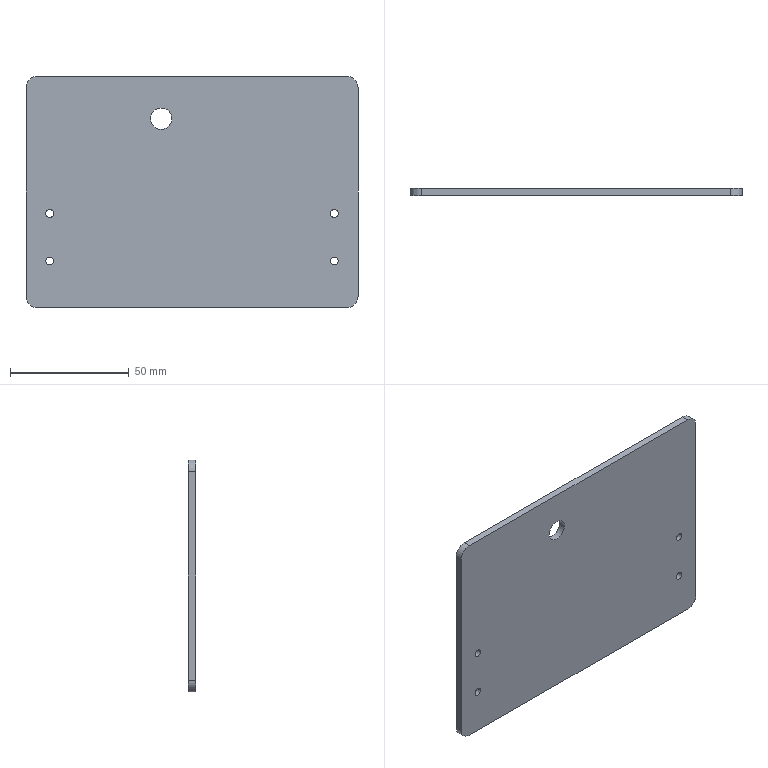Part | NX | 1 solid | 30 faces | box 140 x 3 x 97.8 mm | volume 40712 mm3 | cylinder 14 | cone 10 | plane 6 | commonest cylinder face diameters 3.3 x8 10 x4 9 x2
STEP:
#1=CARTESIAN_POINT('',(1167.,-112.5,-32.3));
#2=VERTEX_POINT('',#1);
#3=CARTESIAN_POINT('',(1167.,-109.5,-32.3));
#4=VERTEX_POINT('',#3);
#5=CARTESIAN_POINT('',(1167.,-112.5,-32.3));
#6=DIRECTION('',(0.,1.,0.));
#7=VECTOR('',#6,1000.);
#8=LINE('',#5,#7);
#9=EDGE_CURVE('',#2,#4,#8,.T.);
#10=ORIENTED_EDGE('',*,*,#9,.F.);
#11=CARTESIAN_POINT('',(1167.,-112.5,55.5));
#12=VERTEX_POINT('',#11);
#13=CARTESIAN_POINT('',(1167.,-112.5,40.233));
#14=DIRECTION('',(0.,0.,1.));
#15=VECTOR('',#14,1000.);
#16=LINE('',#13,#15);
#17=EDGE_CURVE('',#2,#12,#16,.T.);
#18=ORIENTED_EDGE('',*,*,#17,.T.);
#19=CARTESIAN_POINT('',(1167.,-109.5,55.5));
#20=VERTEX_POINT('',#19);
#21=CARTESIAN_POINT('',(1167.,-112.5,55.5));
#22=DIRECTION('',(0.,1.,0.));
#23=VECTOR('',#22,1000.);
#24=LINE('',#21,#23);
#25=EDGE_CURVE('',#12,#20,#24,.T.);
#26=ORIENTED_EDGE('',*,*,#25,.T.);
#27=CARTESIAN_POINT('',(1167.,-109.5,40.233));
#28=DIRECTION('',(0.,0.,1.));
#29=VECTOR('',#28,1000.);
#30=LINE('',#27,#29);
#31=EDGE_CURVE('',#4,#20,#30,.T.);
#32=ORIENTED_EDGE('',*,*,#31,.F.);
#33=EDGE_LOOP('',(#10,#18,#26,#32));
#34=FACE_BOUND('',#33,.T.);
#35=CARTESIAN_POINT('',(1167.,-112.5,22.3));
#36=DIRECTION('',(-1.,0.,0.));
#37=DIRECTION('',(0.,0.,1.));
#38=AXIS2_PLACEMENT_3D('',#35,#36,#37);
#39=PLANE('',#38);
#40=ADVANCED_FACE('',(#34),#39,.T.);
#41=CARTESIAN_POINT('',(1302.,-109.5,60.5));
#42=VERTEX_POINT('',#41);
#43=CARTESIAN_POINT('',(1302.,-112.5,60.5));
#44=VERTEX_POINT('',#43);
#45=CARTESIAN_POINT('',(1302.,-112.5,60.5));
#46=DIRECTION('',(0.,-1.,0.));
#47=VECTOR('',#46,1000.);
#48=LINE('',#45,#47);
#49=EDGE_CURVE('',#42,#44,#48,.T.);
#50=ORIENTED_EDGE('',*,*,#49,.F.);
#51=CARTESIAN_POINT('',(1172.,-109.5,60.5));
#52=VERTEX_POINT('',#51);
#53=CARTESIAN_POINT('',(1169.667,-109.5,60.5));
#54=DIRECTION('',(1.,0.,0.));
#55=VECTOR('',#54,1000.);
#56=LINE('',#53,#55);
#57=EDGE_CURVE('',#52,#42,#56,.T.);
#58=ORIENTED_EDGE('',*,*,#57,.F.);
#59=CARTESIAN_POINT('',(1172.,-112.5,60.5));
#60=VERTEX_POINT('',#59);
#61=CARTESIAN_POINT('',(1172.,-112.5,60.5));
#62=DIRECTION('',(0.,1.,0.));
#63=VECTOR('',#62,1000.);
#64=LINE('',#61,#63);
#65=EDGE_CURVE('',#60,#52,#64,.T.);
#66=ORIENTED_EDGE('',*,*,#65,.F.);
#67=CARTESIAN_POINT('',(1169.667,-112.5,60.5));
#68=DIRECTION('',(1.,0.,0.));
#69=VECTOR('',#68,1000.);
#70=LINE('',#67,#69);
#71=EDGE_CURVE('',#60,#44,#70,.T.);
#72=ORIENTED_EDGE('',*,*,#71,.T.);
#73=EDGE_LOOP('',(#50,#58,#66,#72));
#74=FACE_BOUND('',#73,.T.);
#75=CARTESIAN_POINT('',(1307.,-112.5,60.5));
#76=DIRECTION('',(0.,0.,1.));
#77=DIRECTION('',(1.,0.,0.));
#78=AXIS2_PLACEMENT_3D('',#75,#76,#77);
#79=PLANE('',#78);
#80=ADVANCED_FACE('',(#74),#79,.T.);
#81=CARTESIAN_POINT('',(1307.,-112.5,-32.3));
#82=VERTEX_POINT('',#81);
#83=CARTESIAN_POINT('',(1307.,-109.5,-32.3));
#84=VERTEX_POINT('',#83);
#85=CARTESIAN_POINT('',(1307.,-112.5,-32.3));
#86=DIRECTION('',(0.,1.,0.));
#87=VECTOR('',#86,1000.);
#88=LINE('',#85,#87);
#89=EDGE_CURVE('',#82,#84,#88,.T.);
#90=ORIENTED_EDGE('',*,*,#89,.T.);
#91=CARTESIAN_POINT('',(1307.,-109.5,55.5));
#92=VERTEX_POINT('',#91);
#93=CARTESIAN_POINT('',(1307.,-109.5,40.233));
#94=DIRECTION('',(0.,0.,1.));
#95=VECTOR('',#94,1000.);
#96=LINE('',#93,#95);
#97=EDGE_CURVE('',#84,#92,#96,.T.);
#98=ORIENTED_EDGE('',*,*,#97,.T.);
#99=CARTESIAN_POINT('',(1307.,-112.5,55.5));
#100=VERTEX_POINT('',#99);
#101=CARTESIAN_POINT('',(1307.,-112.5,55.5));
#102=DIRECTION('',(0.,-1.,0.));
#103=VECTOR('',#102,1000.);
#104=LINE('',#101,#103);
#105=EDGE_CURVE('',#92,#100,#104,.T.);
#106=ORIENTED_EDGE('',*,*,#105,.T.);
#107=CARTESIAN_POINT('',(1307.,-112.5,40.233));
#108=DIRECTION('',(0.,0.,1.));
#109=VECTOR('',#108,1000.);
#110=LINE('',#107,#109);
#111=EDGE_CURVE('',#82,#100,#110,.T.);
#112=ORIENTED_EDGE('',*,*,#111,.F.);
#113=EDGE_LOOP('',(#90,#98,#106,#112));
#114=FACE_BOUND('',#113,.T.);
#115=CARTESIAN_POINT('',(1307.,-112.5,-37.3));
#116=DIRECTION('',(1.,0.,0.));
#117=DIRECTION('',(0.,1.,0.));
#118=AXIS2_PLACEMENT_3D('',#115,#116,#117);
#119=PLANE('',#118);
#120=ADVANCED_FACE('',(#114),#119,.T.);
#121=CARTESIAN_POINT('',(1302.,-112.5,-37.3));
#122=VERTEX_POINT('',#121);
#123=CARTESIAN_POINT('',(1172.,-112.5,-37.3));
#124=VERTEX_POINT('',#123);
#125=CARTESIAN_POINT('',(1307.,-112.5,-37.3));
#126=DIRECTION('',(-1.,0.,0.));
#127=VECTOR('',#126,1000.);
#128=LINE('',#125,#127);
#129=EDGE_CURVE('',#122,#124,#128,.T.);
#130=ORIENTED_EDGE('',*,*,#129,.T.);
#131=CARTESIAN_POINT('',(1172.,-109.5,-37.3));
#132=VERTEX_POINT('',#131);
#133=CARTESIAN_POINT('',(1172.,-112.5,-37.3));
#134=DIRECTION('',(0.,1.,0.));
#135=VECTOR('',#134,1000.);
#136=LINE('',#133,#135);
#137=EDGE_CURVE('',#124,#132,#136,.T.);
#138=ORIENTED_EDGE('',*,*,#137,.T.);
#139=CARTESIAN_POINT('',(1302.,-109.5,-37.3));
#140=VERTEX_POINT('',#139);
#141=CARTESIAN_POINT('',(1307.,-109.5,-37.3));
#142=DIRECTION('',(-1.,0.,0.));
#143=VECTOR('',#142,1000.);
#144=LINE('',#141,#143);
#145=EDGE_CURVE('',#140,#132,#144,.T.);
#146=ORIENTED_EDGE('',*,*,#145,.F.);
#147=CARTESIAN_POINT('',(1302.,-112.5,-37.3));
#148=DIRECTION('',(0.,1.,0.));
#149=VECTOR('',#148,1000.);
#150=LINE('',#147,#149);
#151=EDGE_CURVE('',#122,#140,#150,.T.);
#152=ORIENTED_EDGE('',*,*,#151,.F.);
#153=EDGE_LOOP('',(#130,#138,#146,#152));
#154=FACE_BOUND('',#153,.T.);
#155=CARTESIAN_POINT('',(1167.,-112.5,-37.3));
#156=DIRECTION('',(0.,0.,-1.));
#157=DIRECTION('',(0.,-1.,0.));
#158=AXIS2_PLACEMENT_3D('',#155,#156,#157);
#159=PLANE('',#158);
#160=ADVANCED_FACE('',(#154),#159,.T.);
#161=ORIENTED_EDGE('',*,*,#25,.F.);
#162=CARTESIAN_POINT('',(1172.,-112.5,55.5));
#163=DIRECTION('',(0.,1.,0.));
#164=DIRECTION('',(-1.,0.,0.));
#165=AXIS2_PLACEMENT_3D('',#162,#163,#164);
#166=CIRCLE('',#165,5.);
#167=EDGE_CURVE('',#12,#60,#166,.T.);
#168=ORIENTED_EDGE('',*,*,#167,.T.);
#169=ORIENTED_EDGE('',*,*,#65,.T.);
#170=CARTESIAN_POINT('',(1172.,-109.5,55.5));
#171=DIRECTION('',(0.,1.,0.));
#172=DIRECTION('',(-1.,0.,0.));
#173=AXIS2_PLACEMENT_3D('',#170,#171,#172);
#174=CIRCLE('',#173,5.);
#175=EDGE_CURVE('',#20,#52,#174,.T.);
#176=ORIENTED_EDGE('',*,*,#175,.F.);
#177=EDGE_LOOP('',(#161,#168,#169,#176));
#178=FACE_BOUND('',#177,.T.);
#179=CARTESIAN_POINT('',(1172.,-112.5,55.5));
#180=DIRECTION('',(0.,1.,0.));
#181=DIRECTION('',(-1.,0.,0.));
#182=AXIS2_PLACEMENT_3D('',#179,#180,#181);
#183=CYLINDRICAL_SURFACE('',#182,5.);
#184=ADVANCED_FACE('',(#178),#183,.T.);
#185=ORIENTED_EDGE('',*,*,#49,.T.);
#186=CARTESIAN_POINT('',(1302.,-112.5,55.5));
#187=DIRECTION('',(0.,-1.,0.));
#188=DIRECTION('',(1.,0.,0.));
#189=AXIS2_PLACEMENT_3D('',#186,#187,#188);
#190=CIRCLE('',#189,5.);
#191=EDGE_CURVE('',#100,#44,#190,.T.);
#192=ORIENTED_EDGE('',*,*,#191,.F.);
#193=ORIENTED_EDGE('',*,*,#105,.F.);
#194=CARTESIAN_POINT('',(1302.,-109.5,55.5));
#195=DIRECTION('',(0.,-1.,0.));
#196=DIRECTION('',(1.,0.,0.));
#197=AXIS2_PLACEMENT_3D('',#194,#195,#196);
#198=CIRCLE('',#197,5.);
#199=EDGE_CURVE('',#92,#42,#198,.T.);
#200=ORIENTED_EDGE('',*,*,#199,.T.);
#201=EDGE_LOOP('',(#185,#192,#193,#200));
#202=FACE_BOUND('',#201,.T.);
#203=CARTESIAN_POINT('',(1302.,-112.5,55.5));
#204=DIRECTION('',(0.,-1.,0.));
#205=DIRECTION('',(1.,0.,0.));
#206=AXIS2_PLACEMENT_3D('',#203,#204,#205);
#207=CYLINDRICAL_SURFACE('',#206,5.);
#208=ADVANCED_FACE('',(#202),#207,.T.);
#209=ORIENTED_EDGE('',*,*,#89,.F.);
#210=CARTESIAN_POINT('',(1302.,-112.5,-32.3));
#211=DIRECTION('',(0.,1.,0.));
#212=DIRECTION('',(-1.,0.,0.));
#213=AXIS2_PLACEMENT_3D('',#210,#211,#212);
#214=CIRCLE('',#213,5.);
#215=EDGE_CURVE('',#82,#122,#214,.T.);
#216=ORIENTED_EDGE('',*,*,#215,.T.);
#217=ORIENTED_EDGE('',*,*,#151,.T.);
#218=CARTESIAN_POINT('',(1302.,-109.5,-32.3));
#219=DIRECTION('',(0.,1.,0.));
#220=DIRECTION('',(-1.,0.,0.));
#221=AXIS2_PLACEMENT_3D('',#218,#219,#220);
#222=CIRCLE('',#221,5.);
#223=EDGE_CURVE('',#84,#140,#222,.T.);
#224=ORIENTED_EDGE('',*,*,#223,.F.);
#225=EDGE_LOOP('',(#209,#216,#217,#224));
#226=FACE_BOUND('',#225,.T.);
#227=CARTESIAN_POINT('',(1302.,-112.5,-32.3));
#228=DIRECTION('',(0.,1.,0.));
#229=DIRECTION('',(-1.,0.,0.));
#230=AXIS2_PLACEMENT_3D('',#227,#228,#229);
#231=CYLINDRICAL_SURFACE('',#230,5.);
#232=ADVANCED_FACE('',(#226),#231,.T.);
#233=ORIENTED_EDGE('',*,*,#9,.T.);
#234=CARTESIAN_POINT('',(1172.,-109.5,-32.3));
#235=DIRECTION('',(0.,1.,0.));
#236=DIRECTION('',(-1.,0.,0.));
#237=AXIS2_PLACEMENT_3D('',#234,#235,#236);
#238=CIRCLE('',#237,5.);
#239=EDGE_CURVE('',#132,#4,#238,.T.);
#240=ORIENTED_EDGE('',*,*,#239,.F.);
#241=ORIENTED_EDGE('',*,*,#137,.F.);
#242=CARTESIAN_POINT('',(1172.,-112.5,-32.3));
#243=DIRECTION('',(0.,1.,0.));
#244=DIRECTION('',(-1.,0.,0.));
#245=AXIS2_PLACEMENT_3D('',#242,#243,#244);
#246=CIRCLE('',#245,5.);
#247=EDGE_CURVE('',#124,#2,#246,.T.);
#248=ORIENTED_EDGE('',*,*,#247,.T.);
#249=EDGE_LOOP('',(#233,#240,#241,#248));
#250=FACE_BOUND('',#249,.T.);
#251=CARTESIAN_POINT('',(1172.,-112.5,-32.3));
#252=DIRECTION('',(0.,1.,0.));
#253=DIRECTION('',(-1.,0.,0.));
#254=AXIS2_PLACEMENT_3D('',#251,#252,#253);
#255=CYLINDRICAL_SURFACE('',#254,5.);
#256=ADVANCED_FACE('',(#250),#255,.T.);
#257=CARTESIAN_POINT('',(1178.65,-109.884,-17.5));
#258=VERTEX_POINT('',#257);
#259=CARTESIAN_POINT('',(1175.35,-109.884,-17.5));
#260=VERTEX_POINT('',#259);
#261=CARTESIAN_POINT('',(1177.,-109.884,-17.5));
#262=DIRECTION('',(0.,1.,0.));
#263=DIRECTION('',(-1.,0.,0.));
#264=AXIS2_PLACEMENT_3D('',#261,#262,#263);
#265=CIRCLE('',#264,1.65);
#266=EDGE_CURVE('',#258,#260,#265,.T.);
#267=ORIENTED_EDGE('',*,*,#266,.T.);
#268=CARTESIAN_POINT('',(1175.35,-112.5,-17.5));
#269=VERTEX_POINT('',#268);
#270=CARTESIAN_POINT('',(1175.35,-109.5,-17.5));
#271=DIRECTION('',(0.,1.,0.));
#272=VECTOR('',#271,1000.);
#273=LINE('',#270,#272);
#274=EDGE_CURVE('',#260,#269,#273,.F.);
#275=ORIENTED_EDGE('',*,*,#274,.T.);
#276=CARTESIAN_POINT('',(1178.65,-112.5,-17.5));
#277=VERTEX_POINT('',#276);
#278=CARTESIAN_POINT('',(1177.,-112.5,-17.5));
#279=DIRECTION('',(0.,1.,0.));
#280=DIRECTION('',(-1.,0.,0.));
#281=AXIS2_PLACEMENT_3D('',#278,#279,#280);
#282=CIRCLE('',#281,1.65);
#283=EDGE_CURVE('',#277,#269,#282,.T.);
#284=ORIENTED_EDGE('',*,*,#283,.F.);
#285=CARTESIAN_POINT('',(1178.65,-109.5,-17.5));
#286=DIRECTION('',(0.,1.,0.));
#287=VECTOR('',#286,1000.);
#288=LINE('',#285,#287);
#289=EDGE_CURVE('',#258,#277,#288,.F.);
#290=ORIENTED_EDGE('',*,*,#289,.F.);
#291=EDGE_LOOP('',(#267,#275,#284,#290));
#292=FACE_BOUND('',#291,.T.);
#293=CARTESIAN_POINT('',(1177.,-109.5,-17.5));
#294=DIRECTION('',(0.,1.,0.));
#295=DIRECTION('',(-1.,0.,0.));
#296=AXIS2_PLACEMENT_3D('',#293,#294,#295);
#297=CYLINDRICAL_SURFACE('',#296,1.65);
#298=ADVANCED_FACE('',(#292),#297,.F.);
#299=ORIENTED_EDGE('',*,*,#266,.F.);
#300=CARTESIAN_POINT('',(1179.315,-109.5,-17.5));
#301=VERTEX_POINT('',#300);
#302=CARTESIAN_POINT('',(1178.65,-109.884,-17.5));
#303=DIRECTION('',(0.866,0.5,0.));
#304=VECTOR('',#303,1000.);
#305=LINE('',#302,#304);
#306=EDGE_CURVE('',#301,#258,#305,.F.);
#307=ORIENTED_EDGE('',*,*,#306,.F.);
#308=CARTESIAN_POINT('',(1174.685,-109.5,-17.5));
#309=VERTEX_POINT('',#308);
#310=CARTESIAN_POINT('',(1177.,-109.5,-17.5));
#311=DIRECTION('',(0.,1.,0.));
#312=DIRECTION('',(-1.,0.,0.));
#313=AXIS2_PLACEMENT_3D('',#310,#311,#312);
#314=CIRCLE('',#313,2.315);
#315=EDGE_CURVE('',#301,#309,#314,.T.);
#316=ORIENTED_EDGE('',*,*,#315,.T.);
#317=CARTESIAN_POINT('',(1175.35,-109.884,-17.5));
#318=DIRECTION('',(-0.866,0.5,0.));
#319=VECTOR('',#318,1000.);
#320=LINE('',#317,#319);
#321=EDGE_CURVE('',#309,#260,#320,.F.);
#322=ORIENTED_EDGE('',*,*,#321,.T.);
#323=EDGE_LOOP('',(#299,#307,#316,#322));
#324=FACE_BOUND('',#323,.T.);
#325=CARTESIAN_POINT('',(1177.,-109.884,-17.5));
#326=DIRECTION('',(0.,1.,0.));
#327=DIRECTION('',(-1.,0.,0.));
#328=AXIS2_PLACEMENT_3D('',#325,#326,#327);
#329=CONICAL_SURFACE('',#328,1.65,1.047);
#330=ADVANCED_FACE('',(#324),#329,.F.);
#331=CARTESIAN_POINT('',(1178.65,-109.884,2.5));
#332=VERTEX_POINT('',#331);
#333=CARTESIAN_POINT('',(1175.35,-109.884,2.5));
#334=VERTEX_POINT('',#333);
#335=CARTESIAN_POINT('',(1177.,-109.884,2.5));
#336=DIRECTION('',(0.,1.,0.));
#337=DIRECTION('',(-1.,0.,0.));
#338=AXIS2_PLACEMENT_3D('',#335,#336,#337);
#339=CIRCLE('',#338,1.65);
#340=EDGE_CURVE('',#332,#334,#339,.T.);
#341=ORIENTED_EDGE('',*,*,#340,.T.);
#342=CARTESIAN_POINT('',(1175.35,-112.5,2.5));
#343=VERTEX_POINT('',#342);
#344=CARTESIAN_POINT('',(1175.35,-109.5,2.5));
#345=DIRECTION('',(0.,1.,0.));
#346=VECTOR('',#345,1000.);
#347=LINE('',#344,#346);
#348=EDGE_CURVE('',#334,#343,#347,.F.);
#349=ORIENTED_EDGE('',*,*,#348,.T.);
#350=CARTESIAN_POINT('',(1178.65,-112.5,2.5));
#351=VERTEX_POINT('',#350);
#352=CARTESIAN_POINT('',(1177.,-112.5,2.5));
#353=DIRECTION('',(0.,1.,0.));
#354=DIRECTION('',(-1.,0.,0.));
#355=AXIS2_PLACEMENT_3D('',#352,#353,#354);
#356=CIRCLE('',#355,1.65);
#357=EDGE_CURVE('',#351,#343,#356,.T.);
#358=ORIENTED_EDGE('',*,*,#357,.F.);
#359=CARTESIAN_POINT('',(1178.65,-109.5,2.5));
#360=DIRECTION('',(0.,1.,0.));
#361=VECTOR('',#360,1000.);
#362=LINE('',#359,#361);
#363=EDGE_CURVE('',#332,#351,#362,.F.);
#364=ORIENTED_EDGE('',*,*,#363,.F.);
#365=EDGE_LOOP('',(#341,#349,#358,#364));
#366=FACE_BOUND('',#365,.T.);
#367=CARTESIAN_POINT('',(1177.,-109.5,2.5));
#368=DIRECTION('',(0.,1.,0.));
#369=DIRECTION('',(-1.,0.,0.));
#370=AXIS2_PLACEMENT_3D('',#367,#368,#369);
#371=CYLINDRICAL_SURFACE('',#370,1.65);
#372=ADVANCED_FACE('',(#366),#371,.F.);
#373=ORIENTED_EDGE('',*,*,#340,.F.);
#374=CARTESIAN_POINT('',(1179.315,-109.5,2.5));
#375=VERTEX_POINT('',#374);
#376=CARTESIAN_POINT('',(1178.65,-109.884,2.5));
#377=DIRECTION('',(0.866,0.5,0.));
#378=VECTOR('',#377,1000.);
#379=LINE('',#376,#378);
#380=EDGE_CURVE('',#375,#332,#379,.F.);
#381=ORIENTED_EDGE('',*,*,#380,.F.);
#382=CARTESIAN_POINT('',(1174.685,-109.5,2.5));
#383=VERTEX_POINT('',#382);
#384=CARTESIAN_POINT('',(1177.,-109.5,2.5));
#385=DIRECTION('',(0.,1.,0.));
#386=DIRECTION('',(-1.,0.,0.));
#387=AXIS2_PLACEMENT_3D('',#384,#385,#386);
#388=CIRCLE('',#387,2.315);
#389=EDGE_CURVE('',#375,#383,#388,.T.);
#390=ORIENTED_EDGE('',*,*,#389,.T.);
#391=CARTESIAN_POINT('',(1175.35,-109.884,2.5));
#392=DIRECTION('',(-0.866,0.5,0.));
#393=VECTOR('',#392,1000.);
#394=LINE('',#391,#393);
#395=EDGE_CURVE('',#383,#334,#394,.F.);
#396=ORIENTED_EDGE('',*,*,#395,.T.);
#397=EDGE_LOOP('',(#373,#381,#390,#396));
#398=FACE_BOUND('',#397,.T.);
#399=CARTESIAN_POINT('',(1177.,-109.884,2.5));
#400=DIRECTION('',(0.,1.,0.));
#401=DIRECTION('',(-1.,0.,0.));
#402=AXIS2_PLACEMENT_3D('',#399,#400,#401);
#403=CONICAL_SURFACE('',#402,1.65,1.047);
#404=ADVANCED_FACE('',(#398),#403,.F.);
#405=CARTESIAN_POINT('',(1298.65,-109.884,2.5));
#406=VERTEX_POINT('',#405);
#407=CARTESIAN_POINT('',(1295.35,-109.884,2.5));
#408=VERTEX_POINT('',#407);
#409=CARTESIAN_POINT('',(1297.,-109.884,2.5));
#410=DIRECTION('',(0.,1.,0.));
#411=DIRECTION('',(-1.,0.,0.));
#412=AXIS2_PLACEMENT_3D('',#409,#410,#411);
#413=CIRCLE('',#412,1.65);
#414=EDGE_CURVE('',#406,#408,#413,.T.);
#415=ORIENTED_EDGE('',*,*,#414,.T.);
#416=CARTESIAN_POINT('',(1295.35,-112.5,2.5));
#417=VERTEX_POINT('',#416);
#418=CARTESIAN_POINT('',(1295.35,-109.5,2.5));
#419=DIRECTION('',(0.,1.,0.));
#420=VECTOR('',#419,1000.);
#421=LINE('',#418,#420);
#422=EDGE_CURVE('',#408,#417,#421,.F.);
#423=ORIENTED_EDGE('',*,*,#422,.T.);
#424=CARTESIAN_POINT('',(1298.65,-112.5,2.5));
#425=VERTEX_POINT('',#424);
#426=CARTESIAN_POINT('',(1297.,-112.5,2.5));
#427=DIRECTION('',(0.,1.,0.));
#428=DIRECTION('',(-1.,0.,0.));
#429=AXIS2_PLACEMENT_3D('',#426,#427,#428);
#430=CIRCLE('',#429,1.65);
#431=EDGE_CURVE('',#425,#417,#430,.T.);
#432=ORIENTED_EDGE('',*,*,#431,.F.);
#433=CARTESIAN_POINT('',(1298.65,-109.5,2.5));
#434=DIRECTION('',(0.,1.,0.));
#435=VECTOR('',#434,1000.);
#436=LINE('',#433,#435);
#437=EDGE_CURVE('',#406,#425,#436,.F.);
#438=ORIENTED_EDGE('',*,*,#437,.F.);
#439=EDGE_LOOP('',(#415,#423,#432,#438));
#440=FACE_BOUND('',#439,.T.);
#441=CARTESIAN_POINT('',(1297.,-109.5,2.5));
#442=DIRECTION('',(0.,1.,0.));
#443=DIRECTION('',(-1.,0.,0.));
#444=AXIS2_PLACEMENT_3D('',#441,#442,#443);
#445=CYLINDRICAL_SURFACE('',#444,1.65);
#446=ADVANCED_FACE('',(#440),#445,.F.);
#447=ORIENTED_EDGE('',*,*,#414,.F.);
#448=CARTESIAN_POINT('',(1299.315,-109.5,2.5));
#449=VERTEX_POINT('',#448);
#450=CARTESIAN_POINT('',(1298.65,-109.884,2.5));
#451=DIRECTION('',(0.866,0.5,0.));
#452=VECTOR('',#451,1000.);
#453=LINE('',#450,#452);
#454=EDGE_CURVE('',#449,#406,#453,.F.);
#455=ORIENTED_EDGE('',*,*,#454,.F.);
#456=CARTESIAN_POINT('',(1294.685,-109.5,2.5));
#457=VERTEX_POINT('',#456);
#458=CARTESIAN_POINT('',(1297.,-109.5,2.5));
#459=DIRECTION('',(0.,1.,0.));
#460=DIRECTION('',(-1.,0.,0.));
#461=AXIS2_PLACEMENT_3D('',#458,#459,#460);
#462=CIRCLE('',#461,2.315);
#463=EDGE_CURVE('',#449,#457,#462,.T.);
#464=ORIENTED_EDGE('',*,*,#463,.T.);
#465=CARTESIAN_POINT('',(1295.35,-109.884,2.5));
#466=DIRECTION('',(-0.866,0.5,0.));
#467=VECTOR('',#466,1000.);
#468=LINE('',#465,#467);
#469=EDGE_CURVE('',#457,#408,#468,.F.);
#470=ORIENTED_EDGE('',*,*,#469,.T.);
#471=EDGE_LOOP('',(#447,#455,#464,#470));
#472=FACE_BOUND('',#471,.T.);
#473=CARTESIAN_POINT('',(1297.,-109.884,2.5));
#474=DIRECTION('',(0.,1.,0.));
#475=DIRECTION('',(-1.,0.,0.));
#476=AXIS2_PLACEMENT_3D('',#473,#474,#475);
#477=CONICAL_SURFACE('',#476,1.65,1.047);
#478=ADVANCED_FACE('',(#472),#477,.F.);
#479=CARTESIAN_POINT('',(1298.65,-109.884,-17.5));
#480=VERTEX_POINT('',#479);
#481=CARTESIAN_POINT('',(1295.35,-109.884,-17.5));
#482=VERTEX_POINT('',#481);
#483=CARTESIAN_POINT('',(1297.,-109.884,-17.5));
#484=DIRECTION('',(0.,1.,0.));
#485=DIRECTION('',(-1.,0.,0.));
#486=AXIS2_PLACEMENT_3D('',#483,#484,#485);
#487=CIRCLE('',#486,1.65);
#488=EDGE_CURVE('',#480,#482,#487,.T.);
#489=ORIENTED_EDGE('',*,*,#488,.T.);
#490=CARTESIAN_POINT('',(1295.35,-112.5,-17.5));
#491=VERTEX_POINT('',#490);
#492=CARTESIAN_POINT('',(1295.35,-109.5,-17.5));
#493=DIRECTION('',(0.,1.,0.));
#494=VECTOR('',#493,1000.);
#495=LINE('',#492,#494);
#496=EDGE_CURVE('',#482,#491,#495,.F.);
#497=ORIENTED_EDGE('',*,*,#496,.T.);
#498=CARTESIAN_POINT('',(1298.65,-112.5,-17.5));
#499=VERTEX_POINT('',#498);
#500=CARTESIAN_POINT('',(1297.,-112.5,-17.5));
#501=DIRECTION('',(0.,1.,0.));
#502=DIRECTION('',(-1.,0.,0.));
#503=AXIS2_PLACEMENT_3D('',#500,#501,#502);
#504=CIRCLE('',#503,1.65);
#505=EDGE_CURVE('',#499,#491,#504,.T.);
#506=ORIENTED_EDGE('',*,*,#505,.F.);
#507=CARTESIAN_POINT('',(1298.65,-109.5,-17.5));
#508=DIRECTION('',(0.,1.,0.));
#509=VECTOR('',#508,1000.);
#510=LINE('',#507,#509);
#511=EDGE_CURVE('',#480,#499,#510,.F.);
#512=ORIENTED_EDGE('',*,*,#511,.F.);
#513=EDGE_LOOP('',(#489,#497,#506,#512));
#514=FACE_BOUND('',#513,.T.);
#515=CARTESIAN_POINT('',(1297.,-109.5,-17.5));
#516=DIRECTION('',(0.,1.,0.));
#517=DIRECTION('',(-1.,0.,0.));
#518=AXIS2_PLACEMENT_3D('',#515,#516,#517);
#519=CYLINDRICAL_SURFACE('',#518,1.65);
#520=ADVANCED_FACE('',(#514),#519,.F.);
#521=ORIENTED_EDGE('',*,*,#488,.F.);
#522=CARTESIAN_POINT('',(1299.315,-109.5,-17.5));
#523=VERTEX_POINT('',#522);
#524=CARTESIAN_POINT('',(1298.65,-109.884,-17.5));
#525=DIRECTION('',(0.866,0.5,0.));
#526=VECTOR('',#525,1000.);
#527=LINE('',#524,#526);
#528=EDGE_CURVE('',#523,#480,#527,.F.);
#529=ORIENTED_EDGE('',*,*,#528,.F.);
#530=CARTESIAN_POINT('',(1294.685,-109.5,-17.5));
#531=VERTEX_POINT('',#530);
#532=CARTESIAN_POINT('',(1297.,-109.5,-17.5));
#533=DIRECTION('',(0.,1.,0.));
#534=DIRECTION('',(-1.,0.,0.));
#535=AXIS2_PLACEMENT_3D('',#532,#533,#534);
#536=CIRCLE('',#535,2.315);
#537=EDGE_CURVE('',#523,#531,#536,.T.);
#538=ORIENTED_EDGE('',*,*,#537,.T.);
#539=CARTESIAN_POINT('',(1295.35,-109.884,-17.5));
#540=DIRECTION('',(-0.866,0.5,0.));
#541=VECTOR('',#540,1000.);
#542=LINE('',#539,#541);
#543=EDGE_CURVE('',#531,#482,#542,.F.);
#544=ORIENTED_EDGE('',*,*,#543,.T.);
#545=EDGE_LOOP('',(#521,#529,#538,#544));
#546=FACE_BOUND('',#545,.T.);
#547=CARTESIAN_POINT('',(1297.,-109.884,-17.5));
#548=DIRECTION('',(0.,1.,0.));
#549=DIRECTION('',(-1.,0.,0.));
#550=AXIS2_PLACEMENT_3D('',#547,#548,#549);
#551=CONICAL_SURFACE('',#550,1.65,1.047);
#552=ADVANCED_FACE('',(#546),#551,.F.);
#553=ORIENTED_EDGE('',*,*,#543,.F.);
#554=CARTESIAN_POINT('',(1297.,-109.5,-17.5));
#555=DIRECTION('',(0.,1.,0.));
#556=DIRECTION('',(-1.,0.,0.));
#557=AXIS2_PLACEMENT_3D('',#554,#555,#556);
#558=CIRCLE('',#557,2.315);
#559=EDGE_CURVE('',#531,#523,#558,.T.);
#560=ORIENTED_EDGE('',*,*,#559,.T.);
#561=ORIENTED_EDGE('',*,*,#528,.T.);
#562=CARTESIAN_POINT('',(1297.,-109.884,-17.5));
#563=DIRECTION('',(0.,1.,0.));
#564=DIRECTION('',(-1.,0.,0.));
#565=AXIS2_PLACEMENT_3D('',#562,#563,#564);
#566=CIRCLE('',#565,1.65);
#567=EDGE_CURVE('',#482,#480,#566,.T.);
#568=ORIENTED_EDGE('',*,*,#567,.F.);
#569=EDGE_LOOP('',(#553,#560,#561,#568));
#570=FACE_BOUND('',#569,.T.);
#571=CARTESIAN_POINT('',(1297.,-109.884,-17.5));
#572=DIRECTION('',(0.,1.,0.));
#573=DIRECTION('',(-1.,0.,0.));
#574=AXIS2_PLACEMENT_3D('',#571,#572,#573);
#575=CONICAL_SURFACE('',#574,1.65,1.047);
#576=ADVANCED_FACE('',(#570),#575,.F.);
#577=ORIENTED_EDGE('',*,*,#348,.F.);
#578=CARTESIAN_POINT('',(1177.,-109.884,2.5));
#579=DIRECTION('',(0.,1.,0.));
#580=DIRECTION('',(-1.,0.,0.));
#581=AXIS2_PLACEMENT_3D('',#578,#579,#580);
#582=CIRCLE('',#581,1.65);
#583=EDGE_CURVE('',#334,#332,#582,.T.);
#584=ORIENTED_EDGE('',*,*,#583,.T.);
#585=ORIENTED_EDGE('',*,*,#363,.T.);
#586=CARTESIAN_POINT('',(1177.,-112.5,2.5));
#587=DIRECTION('',(0.,1.,0.));
#588=DIRECTION('',(-1.,0.,0.));
#589=AXIS2_PLACEMENT_3D('',#586,#587,#588);
#590=CIRCLE('',#589,1.65);
#591=EDGE_CURVE('',#343,#351,#590,.T.);
#592=ORIENTED_EDGE('',*,*,#591,.F.);
#593=EDGE_LOOP('',(#577,#584,#585,#592));
#594=FACE_BOUND('',#593,.T.);
#595=CARTESIAN_POINT('',(1177.,-109.5,2.5));
#596=DIRECTION('',(0.,1.,0.));
#597=DIRECTION('',(-1.,0.,0.));
#598=AXIS2_PLACEMENT_3D('',#595,#596,#597);
#599=CYLINDRICAL_SURFACE('',#598,1.65);
#600=ADVANCED_FACE('',(#594),#599,.F.);
#601=ORIENTED_EDGE('',*,*,#321,.F.);
#602=CARTESIAN_POINT('',(1177.,-109.5,-17.5));
#603=DIRECTION('',(0.,1.,0.));
#604=DIRECTION('',(-1.,0.,0.));
#605=AXIS2_PLACEMENT_3D('',#602,#603,#604);
#606=CIRCLE('',#605,2.315);
#607=EDGE_CURVE('',#309,#301,#606,.T.);
#608=ORIENTED_EDGE('',*,*,#607,.T.);
#609=ORIENTED_EDGE('',*,*,#306,.T.);
#610=CARTESIAN_POINT('',(1177.,-109.884,-17.5));
#611=DIRECTION('',(0.,1.,0.));
#612=DIRECTION('',(-1.,0.,0.));
#613=AXIS2_PLACEMENT_3D('',#610,#611,#612);
#614=CIRCLE('',#613,1.65);
#615=EDGE_CURVE('',#260,#258,#614,.T.);
#616=ORIENTED_EDGE('',*,*,#615,.F.);
#617=EDGE_LOOP('',(#601,#608,#609,#616));
#618=FACE_BOUND('',#617,.T.);
#619=CARTESIAN_POINT('',(1177.,-109.884,-17.5));
#620=DIRECTION('',(0.,1.,0.));
#621=DIRECTION('',(-1.,0.,0.));
#622=AXIS2_PLACEMENT_3D('',#619,#620,#621);
#623=CONICAL_SURFACE('',#622,1.65,1.047);
#624=ADVANCED_FACE('',(#618),#623,.F.);
#625=ORIENTED_EDGE('',*,*,#496,.F.);
#626=ORIENTED_EDGE('',*,*,#567,.T.);
#627=ORIENTED_EDGE('',*,*,#511,.T.);
#628=CARTESIAN_POINT('',(1297.,-112.5,-17.5));
#629=DIRECTION('',(0.,1.,0.));
#630=DIRECTION('',(-1.,0.,0.));
#631=AXIS2_PLACEMENT_3D('',#628,#629,#630);
#632=CIRCLE('',#631,1.65);
#633=EDGE_CURVE('',#491,#499,#632,.T.);
#634=ORIENTED_EDGE('',*,*,#633,.F.);
#635=EDGE_LOOP('',(#625,#626,#627,#634));
#636=FACE_BOUND('',#635,.T.);
#637=CARTESIAN_POINT('',(1297.,-109.5,-17.5));
#638=DIRECTION('',(0.,1.,0.));
#639=DIRECTION('',(-1.,0.,0.));
#640=AXIS2_PLACEMENT_3D('',#637,#638,#639);
#641=CYLINDRICAL_SURFACE('',#640,1.65);
#642=ADVANCED_FACE('',(#636),#641,.F.);
#643=ORIENTED_EDGE('',*,*,#469,.F.);
#644=CARTESIAN_POINT('',(1297.,-109.5,2.5));
#645=DIRECTION('',(0.,1.,0.));
#646=DIRECTION('',(-1.,0.,0.));
#647=AXIS2_PLACEMENT_3D('',#644,#645,#646);
#648=CIRCLE('',#647,2.315);
#649=EDGE_CURVE('',#457,#449,#648,.T.);
#650=ORIENTED_EDGE('',*,*,#649,.T.);
#651=ORIENTED_EDGE('',*,*,#454,.T.);
#652=CARTESIAN_POINT('',(1297.,-109.884,2.5));
#653=DIRECTION('',(0.,1.,0.));
#654=DIRECTION('',(-1.,0.,0.));
#655=AXIS2_PLACEMENT_3D('',#652,#653,#654);
#656=CIRCLE('',#655,1.65);
#657=EDGE_CURVE('',#408,#406,#656,.T.);
#658=ORIENTED_EDGE('',*,*,#657,.F.);
#659=EDGE_LOOP('',(#643,#650,#651,#658));
#660=FACE_BOUND('',#659,.T.);
#661=CARTESIAN_POINT('',(1297.,-109.884,2.5));
#662=DIRECTION('',(0.,1.,0.));
#663=DIRECTION('',(-1.,0.,0.));
#664=AXIS2_PLACEMENT_3D('',#661,#662,#663);
#665=CONICAL_SURFACE('',#664,1.65,1.047);
#666=ADVANCED_FACE('',(#660),#665,.F.);
#667=ORIENTED_EDGE('',*,*,#274,.F.);
#668=ORIENTED_EDGE('',*,*,#615,.T.);
#669=ORIENTED_EDGE('',*,*,#289,.T.);
#670=CARTESIAN_POINT('',(1177.,-112.5,-17.5));
#671=DIRECTION('',(0.,1.,0.));
#672=DIRECTION('',(-1.,0.,0.));
#673=AXIS2_PLACEMENT_3D('',#670,#671,#672);
#674=CIRCLE('',#673,1.65);
#675=EDGE_CURVE('',#269,#277,#674,.T.);
#676=ORIENTED_EDGE('',*,*,#675,.F.);
#677=EDGE_LOOP('',(#667,#668,#669,#676));
#678=FACE_BOUND('',#677,.T.);
#679=CARTESIAN_POINT('',(1177.,-109.5,-17.5));
#680=DIRECTION('',(0.,1.,0.));
#681=DIRECTION('',(-1.,0.,0.));
#682=AXIS2_PLACEMENT_3D('',#679,#680,#681);
#683=CYLINDRICAL_SURFACE('',#682,1.65);
#684=ADVANCED_FACE('',(#678),#683,.F.);
#685=ORIENTED_EDGE('',*,*,#422,.F.);
#686=ORIENTED_EDGE('',*,*,#657,.T.);
#687=ORIENTED_EDGE('',*,*,#437,.T.);
#688=CARTESIAN_POINT('',(1297.,-112.5,2.5));
#689=DIRECTION('',(0.,1.,0.));
#690=DIRECTION('',(-1.,0.,0.));
#691=AXIS2_PLACEMENT_3D('',#688,#689,#690);
#692=CIRCLE('',#691,1.65);
#693=EDGE_CURVE('',#417,#425,#692,.T.);
#694=ORIENTED_EDGE('',*,*,#693,.F.);
#695=EDGE_LOOP('',(#685,#686,#687,#694));
#696=FACE_BOUND('',#695,.T.);
#697=CARTESIAN_POINT('',(1297.,-109.5,2.5));
#698=DIRECTION('',(0.,1.,0.));
#699=DIRECTION('',(-1.,0.,0.));
#700=AXIS2_PLACEMENT_3D('',#697,#698,#699);
#701=CYLINDRICAL_SURFACE('',#700,1.65);
#702=ADVANCED_FACE('',(#696),#701,.F.);
#703=ORIENTED_EDGE('',*,*,#395,.F.);
#704=CARTESIAN_POINT('',(1177.,-109.5,2.5));
#705=DIRECTION('',(0.,1.,0.));
#706=DIRECTION('',(-1.,0.,0.));
#707=AXIS2_PLACEMENT_3D('',#704,#705,#706);
#708=CIRCLE('',#707,2.315);
#709=EDGE_CURVE('',#383,#375,#708,.T.);
#710=ORIENTED_EDGE('',*,*,#709,.T.);
#711=ORIENTED_EDGE('',*,*,#380,.T.);
#712=ORIENTED_EDGE('',*,*,#583,.F.);
#713=EDGE_LOOP('',(#703,#710,#711,#712));
#714=FACE_BOUND('',#713,.T.);
#715=CARTESIAN_POINT('',(1177.,-109.884,2.5));
#716=DIRECTION('',(0.,1.,0.));
#717=DIRECTION('',(-1.,0.,0.));
#718=AXIS2_PLACEMENT_3D('',#715,#716,#717);
#719=CONICAL_SURFACE('',#718,1.65,1.047);
#720=ADVANCED_FACE('',(#714),#719,.F.);
#721=ORIENTED_EDGE('',*,*,#31,.T.);
#722=ORIENTED_EDGE('',*,*,#175,.T.);
#723=ORIENTED_EDGE('',*,*,#57,.T.);
#724=ORIENTED_EDGE('',*,*,#199,.F.);
#725=ORIENTED_EDGE('',*,*,#97,.F.);
#726=ORIENTED_EDGE('',*,*,#223,.T.);
#727=ORIENTED_EDGE('',*,*,#145,.T.);
#728=ORIENTED_EDGE('',*,*,#239,.T.);
#729=EDGE_LOOP('',(#721,#722,#723,#724,#725,#726,#727,#728));
#730=FACE_BOUND('',#729,.T.);
#731=ORIENTED_EDGE('',*,*,#315,.F.);
#732=ORIENTED_EDGE('',*,*,#607,.F.);
#733=EDGE_LOOP('',(#731,#732));
#734=FACE_BOUND('',#733,.T.);
#735=ORIENTED_EDGE('',*,*,#463,.F.);
#736=ORIENTED_EDGE('',*,*,#649,.F.);
#737=EDGE_LOOP('',(#735,#736));
#738=FACE_BOUND('',#737,.T.);
#739=CARTESIAN_POINT('',(1228.7,-109.5,42.5));
#740=VERTEX_POINT('',#739);
#741=CARTESIAN_POINT('',(1219.3,-109.5,42.5));
#742=VERTEX_POINT('',#741);
#743=CARTESIAN_POINT('',(1224.,-109.5,42.5));
#744=DIRECTION('',(0.,1.,0.));
#745=DIRECTION('',(-1.,0.,0.));
#746=AXIS2_PLACEMENT_3D('',#743,#744,#745);
#747=CIRCLE('',#746,4.7);
#748=EDGE_CURVE('',#740,#742,#747,.T.);
#749=ORIENTED_EDGE('',*,*,#748,.F.);
#750=CARTESIAN_POINT('',(1224.,-109.5,42.5));
#751=DIRECTION('',(0.,1.,0.));
#752=DIRECTION('',(-1.,0.,0.));
#753=AXIS2_PLACEMENT_3D('',#750,#751,#752);
#754=CIRCLE('',#753,4.7);
#755=EDGE_CURVE('',#742,#740,#754,.T.);
#756=ORIENTED_EDGE('',*,*,#755,.F.);
#757=EDGE_LOOP('',(#749,#756));
#758=FACE_BOUND('',#757,.T.);
#759=ORIENTED_EDGE('',*,*,#537,.F.);
#760=ORIENTED_EDGE('',*,*,#559,.F.);
#761=EDGE_LOOP('',(#759,#760));
#762=FACE_BOUND('',#761,.T.);
#763=ORIENTED_EDGE('',*,*,#389,.F.);
#764=ORIENTED_EDGE('',*,*,#709,.F.);
#765=EDGE_LOOP('',(#763,#764));
#766=FACE_BOUND('',#765,.T.);
#767=CARTESIAN_POINT('',(1169.667,-109.5,40.233));
#768=DIRECTION('',(0.,1.,0.));
#769=DIRECTION('',(1.,0.,0.));
#770=AXIS2_PLACEMENT_3D('',#767,#768,#769);
#771=PLANE('',#770);
#772=ADVANCED_FACE('',(#730,#734,#738,#758,#762,#766),#771,.T.);
#773=CARTESIAN_POINT('',(1228.5,-109.7,42.5));
#774=VERTEX_POINT('',#773);
#775=CARTESIAN_POINT('',(1219.5,-109.7,42.5));
#776=VERTEX_POINT('',#775);
#777=CARTESIAN_POINT('',(1224.,-109.7,42.5));
#778=DIRECTION('',(0.,1.,0.));
#779=DIRECTION('',(-1.,0.,0.));
#780=AXIS2_PLACEMENT_3D('',#777,#778,#779);
#781=CIRCLE('',#780,4.5);
#782=EDGE_CURVE('',#774,#776,#781,.T.);
#783=ORIENTED_EDGE('',*,*,#782,.T.);
#784=CARTESIAN_POINT('',(1219.5,-112.5,42.5));
#785=VERTEX_POINT('',#784);
#786=CARTESIAN_POINT('',(1219.5,-109.5,42.5));
#787=DIRECTION('',(0.,1.,0.));
#788=VECTOR('',#787,1000.);
#789=LINE('',#786,#788);
#790=EDGE_CURVE('',#776,#785,#789,.F.);
#791=ORIENTED_EDGE('',*,*,#790,.T.);
#792=CARTESIAN_POINT('',(1228.5,-112.5,42.5));
#793=VERTEX_POINT('',#792);
#794=CARTESIAN_POINT('',(1224.,-112.5,42.5));
#795=DIRECTION('',(0.,1.,0.));
#796=DIRECTION('',(-1.,0.,0.));
#797=AXIS2_PLACEMENT_3D('',#794,#795,#796);
#798=CIRCLE('',#797,4.5);
#799=EDGE_CURVE('',#793,#785,#798,.T.);
#800=ORIENTED_EDGE('',*,*,#799,.F.);
#801=CARTESIAN_POINT('',(1228.5,-109.5,42.5));
#802=DIRECTION('',(0.,1.,0.));
#803=VECTOR('',#802,1000.);
#804=LINE('',#801,#803);
#805=EDGE_CURVE('',#774,#793,#804,.F.);
#806=ORIENTED_EDGE('',*,*,#805,.F.);
#807=EDGE_LOOP('',(#783,#791,#800,#806));
#808=FACE_BOUND('',#807,.T.);
#809=CARTESIAN_POINT('',(1224.,-109.5,42.5));
#810=DIRECTION('',(0.,1.,0.));
#811=DIRECTION('',(-1.,0.,0.));
#812=AXIS2_PLACEMENT_3D('',#809,#810,#811);
#813=CYLINDRICAL_SURFACE('',#812,4.5);
#814=ADVANCED_FACE('',(#808),#813,.F.);
#815=ORIENTED_EDGE('',*,*,#782,.F.);
#816=CARTESIAN_POINT('',(1228.5,-109.7,42.5));
#817=DIRECTION('',(0.7071,0.7071,0.));
#818=VECTOR('',#817,1000.);
#819=LINE('',#816,#818);
#820=EDGE_CURVE('',#740,#774,#819,.F.);
#821=ORIENTED_EDGE('',*,*,#820,.F.);
#822=ORIENTED_EDGE('',*,*,#748,.T.);
#823=CARTESIAN_POINT('',(1219.5,-109.7,42.5));
#824=DIRECTION('',(-0.7071,0.7071,0.));
#825=VECTOR('',#824,1000.);
#826=LINE('',#823,#825);
#827=EDGE_CURVE('',#742,#776,#826,.F.);
#828=ORIENTED_EDGE('',*,*,#827,.T.);
#829=EDGE_LOOP('',(#815,#821,#822,#828));
#830=FACE_BOUND('',#829,.T.);
#831=CARTESIAN_POINT('',(1224.,-109.7,42.5));
#832=DIRECTION('',(0.,1.,0.));
#833=DIRECTION('',(-1.,0.,0.));
#834=AXIS2_PLACEMENT_3D('',#831,#832,#833);
#835=CONICAL_SURFACE('',#834,4.5,0.7854);
#836=ADVANCED_FACE('',(#830),#835,.F.);
#837=ORIENTED_EDGE('',*,*,#790,.F.);
#838=CARTESIAN_POINT('',(1224.,-109.7,42.5));
#839=DIRECTION('',(0.,1.,0.));
#840=DIRECTION('',(-1.,0.,0.));
#841=AXIS2_PLACEMENT_3D('',#838,#839,#840);
#842=CIRCLE('',#841,4.5);
#843=EDGE_CURVE('',#776,#774,#842,.T.);
#844=ORIENTED_EDGE('',*,*,#843,.T.);
#845=ORIENTED_EDGE('',*,*,#805,.T.);
#846=CARTESIAN_POINT('',(1224.,-112.5,42.5));
#847=DIRECTION('',(0.,1.,0.));
#848=DIRECTION('',(-1.,0.,0.));
#849=AXIS2_PLACEMENT_3D('',#846,#847,#848);
#850=CIRCLE('',#849,4.5);
#851=EDGE_CURVE('',#785,#793,#850,.T.);
#852=ORIENTED_EDGE('',*,*,#851,.F.);
#853=EDGE_LOOP('',(#837,#844,#845,#852));
#854=FACE_BOUND('',#853,.T.);
#855=CARTESIAN_POINT('',(1224.,-109.5,42.5));
#856=DIRECTION('',(0.,1.,0.));
#857=DIRECTION('',(-1.,0.,0.));
#858=AXIS2_PLACEMENT_3D('',#855,#856,#857);
#859=CYLINDRICAL_SURFACE('',#858,4.5);
#860=ADVANCED_FACE('',(#854),#859,.F.);
#861=ORIENTED_EDGE('',*,*,#827,.F.);
#862=ORIENTED_EDGE('',*,*,#755,.T.);
#863=ORIENTED_EDGE('',*,*,#820,.T.);
#864=ORIENTED_EDGE('',*,*,#843,.F.);
#865=EDGE_LOOP('',(#861,#862,#863,#864));
#866=FACE_BOUND('',#865,.T.);
#867=CARTESIAN_POINT('',(1224.,-109.7,42.5));
#868=DIRECTION('',(0.,1.,0.));
#869=DIRECTION('',(-1.,0.,0.));
#870=AXIS2_PLACEMENT_3D('',#867,#868,#869);
#871=CONICAL_SURFACE('',#870,4.5,0.7854);
#872=ADVANCED_FACE('',(#866),#871,.F.);
#873=ORIENTED_EDGE('',*,*,#129,.F.);
#874=ORIENTED_EDGE('',*,*,#215,.F.);
#875=ORIENTED_EDGE('',*,*,#111,.T.);
#876=ORIENTED_EDGE('',*,*,#191,.T.);
#877=ORIENTED_EDGE('',*,*,#71,.F.);
#878=ORIENTED_EDGE('',*,*,#167,.F.);
#879=ORIENTED_EDGE('',*,*,#17,.F.);
#880=ORIENTED_EDGE('',*,*,#247,.F.);
#881=EDGE_LOOP('',(#873,#874,#875,#876,#877,#878,#879,#880));
#882=FACE_BOUND('',#881,.T.);
#883=ORIENTED_EDGE('',*,*,#799,.T.);
#884=ORIENTED_EDGE('',*,*,#851,.T.);
#885=EDGE_LOOP('',(#883,#884));
#886=FACE_BOUND('',#885,.T.);
#887=ORIENTED_EDGE('',*,*,#283,.T.);
#888=ORIENTED_EDGE('',*,*,#675,.T.);
#889=EDGE_LOOP('',(#887,#888));
#890=FACE_BOUND('',#889,.T.);
#891=ORIENTED_EDGE('',*,*,#357,.T.);
#892=ORIENTED_EDGE('',*,*,#591,.T.);
#893=EDGE_LOOP('',(#891,#892));
#894=FACE_BOUND('',#893,.T.);
#895=ORIENTED_EDGE('',*,*,#431,.T.);
#896=ORIENTED_EDGE('',*,*,#693,.T.);
#897=EDGE_LOOP('',(#895,#896));
#898=FACE_BOUND('',#897,.T.);
#899=ORIENTED_EDGE('',*,*,#505,.T.);
#900=ORIENTED_EDGE('',*,*,#633,.T.);
#901=EDGE_LOOP('',(#899,#900));
#902=FACE_BOUND('',#901,.T.);
#903=CARTESIAN_POINT('',(1169.667,-112.5,40.233));
#904=DIRECTION('',(0.,1.,0.));
#905=DIRECTION('',(1.,0.,0.));
#906=AXIS2_PLACEMENT_3D('',#903,#904,#905);
#907=PLANE('',#906);
#908=ADVANCED_FACE('',(#882,#886,#890,#894,#898,#902),#907,.F.);
#909=CLOSED_SHELL('',(#40,#80,#120,#160,#184,#208,#232,#256,#298,#330,#372,#404,#446,#478,#520,#552,#576,#600,#624,#642,#666,#684,#702,#720,#772,#814,#836,#860,#872,#908));
#910=MANIFOLD_SOLID_BREP('',#909);
#911=(LENGTH_UNIT()NAMED_UNIT(*)SI_UNIT(.MILLI.,.METRE.));
#912=UNCERTAINTY_MEASURE_WITH_UNIT(LENGTH_MEASURE(0.00001),#911,'','');
#913=(NAMED_UNIT(*)PLANE_ANGLE_UNIT()SI_UNIT($,.RADIAN.));
#914=(NAMED_UNIT(*)SI_UNIT($,.STERADIAN.)SOLID_ANGLE_UNIT());
#915=(GEOMETRIC_REPRESENTATION_CONTEXT(3)GLOBAL_UNCERTAINTY_ASSIGNED_CONTEXT((#912))GLOBAL_UNIT_ASSIGNED_CONTEXT((#911,#913,#914))REPRESENTATION_CONTEXT('',''));
#916=ADVANCED_BREP_SHAPE_REPRESENTATION('',(#910),#915);